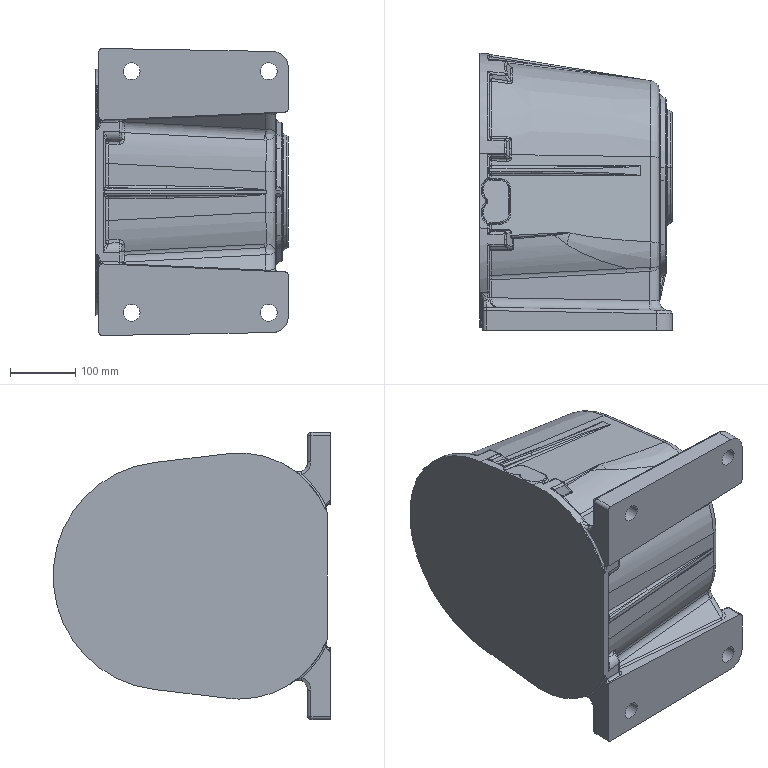Part | STEP file | Input 99 | 1 solid | 615 faces | box 295 x 425 x 439.824 mm | volume 31332402 mm3 | spline 270 | cylinder 180 | plane 89 | torus 33 | sphere 29 | cone 14 | commonest cylinder face diameters 8 x49 6 x36 10 x20 4 x19 30 x18 26 x8